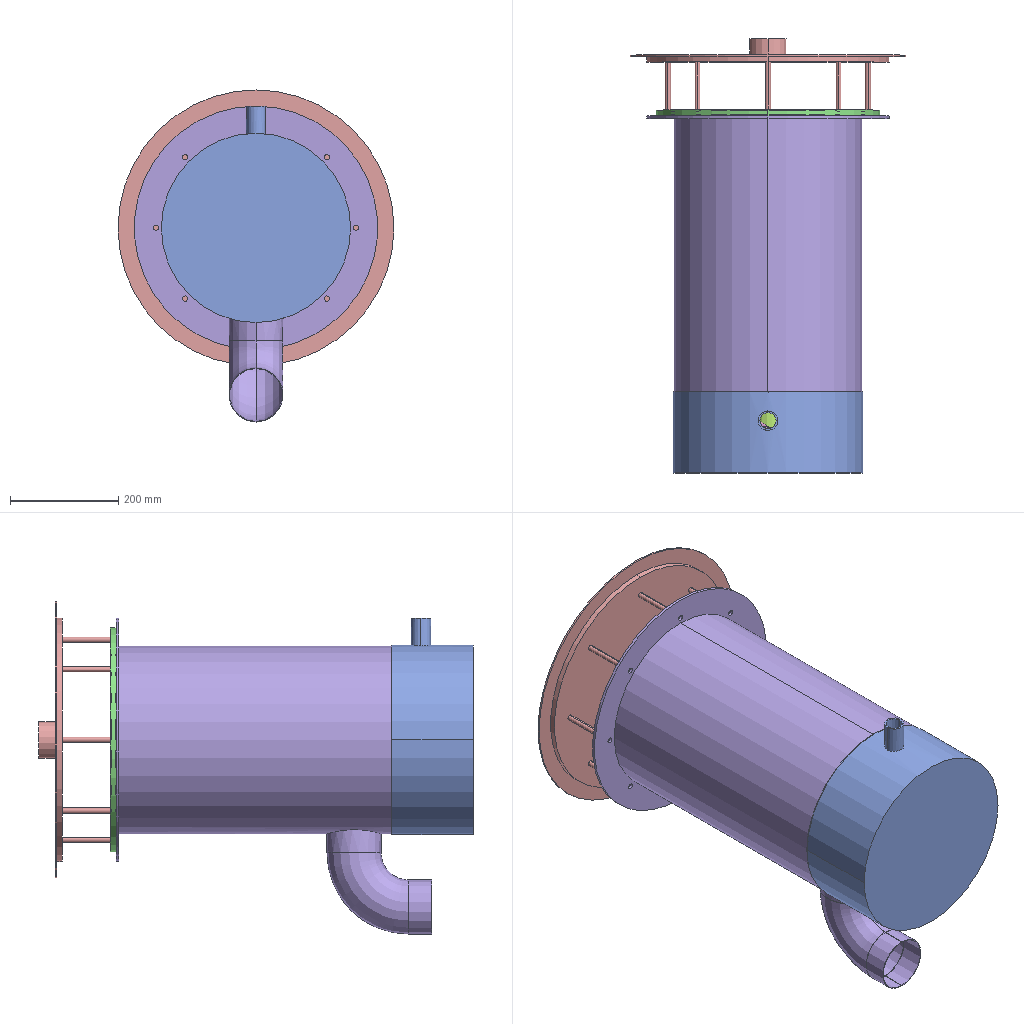Assembly | SolidWorks | 5 different items | 5 placed | box 510 x 803 x 614 mm
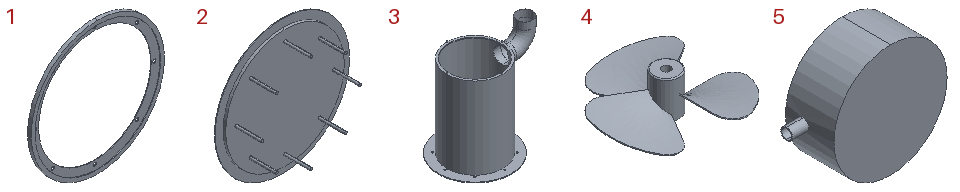Parts list (item | quantity | size | volume | features):
1 | x1 | 414 x 11 x 414 mm | 123980 mm3 | features ICE 2, Extrusion 1
2 | x1 | 510 x 143 x 510 mm | 2374097 mm3 | features ICE 3, Extrusion 1
3 | x1 | 583.992 x 450 x 583.584 mm | 3138291 mm3 | features ICE 5, Cut 2, RefAxis 1, Sweep 1
4 | x1 | 245.378 x 245.378 x 70 mm | 192980 mm3 | features Fillet 2, CirPattern 1, Extrusion 1, Helix 1, RefAxis 1, SweepRefSurface 1, Thicken 1
5 | x1 | 400 x 150 x 350 mm | 1908298 mm3 | features ICE 6, Extrusion 1, Shell 1
Mates (type | each side: item.copy, entity, surface, feature):
Concentric | 5.1 face cylinder Boss-Extrude2 | 3.1 face cylinder Boss-Extrude2
Concentric | 2.1 face cylinder Boss-Extrude6 | 3.1 face cylinder Boss-Extrude2
Coincident | 5.1 face plane Boss-Extrude2 | 3.1 face plane Boss-Extrude5
Concentric | 5.1 face cylinder Boss-Extrude6 | 4.1 face cylinder Boss-Extrude1
Coincident | 5.1 face plane Boss-Extrude3 | 4.1 face plane Boss-Extrude1
Parallel | 5.1 face cylinder Boss-Extrude5 | 3.1 face cylinder Sweep-Thin1
Concentric | 3.1 face cylinder Boss-Extrude4 | 1.1 face cylinder Boss-Extrude2
Coincident | 3.1 face plane Boss-Extrude3 | 1.1 face plane Boss-Extrude3